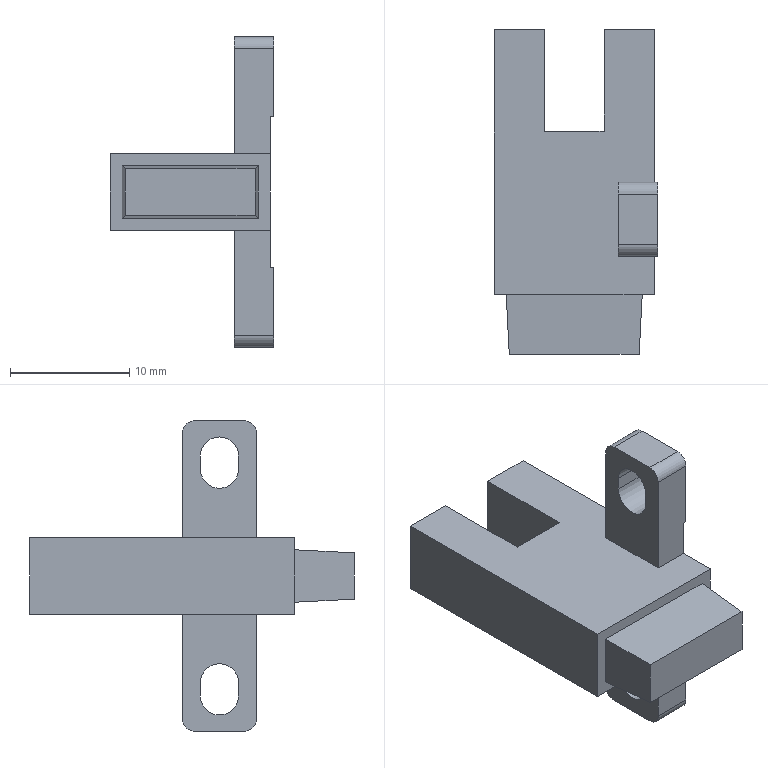Part | STEP file | 0230_015_FPMT54 | 1 solid | 41 faces | box 13.7 x 27.2 x 26 mm | volume 2173 mm3 | plane 31 | cylinder 10 | commonest cylinder face diameters 3.2 x6 2 x4